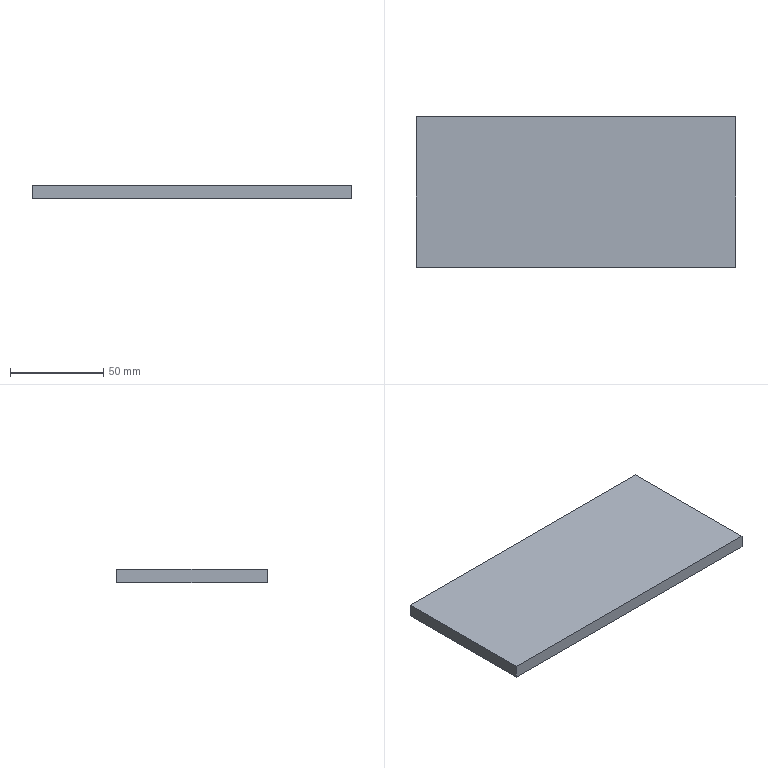Part | STEP file | 2026.6.15-Main Assembly图.sldasm-Part-108 | 1 solid | 6 faces | box 170.9 x 80.5 x 7 mm | volume 96302 mm3 | plane 6
STEP:
#1=CARTESIAN_POINT('',(-1674.674,519.051,4125.667));
#2=VERTEX_POINT('',#1);
#3=CARTESIAN_POINT('',(-1674.674,599.551,4125.667));
#4=VERTEX_POINT('',#3);
#5=CARTESIAN_POINT('',(-1674.674,519.051,4125.667));
#6=DIRECTION('',(0.,1.,0.));
#7=VECTOR('',#6,1000.);
#8=LINE('',#5,#7);
#9=EDGE_CURVE('',#2,#4,#8,.T.);
#10=ORIENTED_EDGE('',*,*,#9,.T.);
#11=CARTESIAN_POINT('',(-1674.674,599.551,4118.667));
#12=VERTEX_POINT('',#11);
#13=CARTESIAN_POINT('',(-1674.674,599.551,4118.667));
#14=DIRECTION('',(0.,0.,1.));
#15=VECTOR('',#14,1000.);
#16=LINE('',#13,#15);
#17=EDGE_CURVE('',#12,#4,#16,.T.);
#18=ORIENTED_EDGE('',*,*,#17,.F.);
#19=CARTESIAN_POINT('',(-1674.674,519.051,4118.667));
#20=VERTEX_POINT('',#19);
#21=CARTESIAN_POINT('',(-1674.674,519.051,4118.667));
#22=DIRECTION('',(0.,1.,0.));
#23=VECTOR('',#22,1000.);
#24=LINE('',#21,#23);
#25=EDGE_CURVE('',#20,#12,#24,.T.);
#26=ORIENTED_EDGE('',*,*,#25,.F.);
#27=CARTESIAN_POINT('',(-1674.674,519.051,4118.667));
#28=DIRECTION('',(0.,0.,1.));
#29=VECTOR('',#28,1000.);
#30=LINE('',#27,#29);
#31=EDGE_CURVE('',#20,#2,#30,.T.);
#32=ORIENTED_EDGE('',*,*,#31,.T.);
#33=EDGE_LOOP('',(#10,#18,#26,#32));
#34=FACE_OUTER_BOUND('',#33,.T.);
#35=CARTESIAN_POINT('',(-1674.674,519.051,4118.667));
#36=DIRECTION('',(1.,0.,0.));
#37=DIRECTION('',(0.,1.,0.));
#38=AXIS2_PLACEMENT_3D('',#35,#36,#37);
#39=PLANE('',#38);
#40=ADVANCED_FACE('',(#34),#39,.F.);
#41=CARTESIAN_POINT('',(-1503.774,599.551,4125.667));
#42=VERTEX_POINT('',#41);
#43=CARTESIAN_POINT('',(-1674.674,599.551,4125.667));
#44=DIRECTION('',(1.,0.,0.));
#45=VECTOR('',#44,1000.);
#46=LINE('',#43,#45);
#47=EDGE_CURVE('',#4,#42,#46,.T.);
#48=ORIENTED_EDGE('',*,*,#47,.T.);
#49=CARTESIAN_POINT('',(-1503.774,599.551,4118.667));
#50=VERTEX_POINT('',#49);
#51=CARTESIAN_POINT('',(-1503.774,599.551,4118.667));
#52=DIRECTION('',(0.,0.,1.));
#53=VECTOR('',#52,1000.);
#54=LINE('',#51,#53);
#55=EDGE_CURVE('',#50,#42,#54,.T.);
#56=ORIENTED_EDGE('',*,*,#55,.F.);
#57=CARTESIAN_POINT('',(-1674.674,599.551,4118.667));
#58=DIRECTION('',(1.,0.,0.));
#59=VECTOR('',#58,1000.);
#60=LINE('',#57,#59);
#61=EDGE_CURVE('',#12,#50,#60,.T.);
#62=ORIENTED_EDGE('',*,*,#61,.F.);
#63=ORIENTED_EDGE('',*,*,#17,.T.);
#64=EDGE_LOOP('',(#48,#56,#62,#63));
#65=FACE_OUTER_BOUND('',#64,.T.);
#66=CARTESIAN_POINT('',(-1674.674,599.551,4118.667));
#67=DIRECTION('',(0.,-1.,0.));
#68=DIRECTION('',(0.,0.,-1.));
#69=AXIS2_PLACEMENT_3D('',#66,#67,#68);
#70=PLANE('',#69);
#71=ADVANCED_FACE('',(#65),#70,.F.);
#72=CARTESIAN_POINT('',(-1503.774,519.051,4125.667));
#73=VERTEX_POINT('',#72);
#74=CARTESIAN_POINT('',(-1503.774,599.551,4125.667));
#75=DIRECTION('',(0.,-1.,0.));
#76=VECTOR('',#75,1000.);
#77=LINE('',#74,#76);
#78=EDGE_CURVE('',#42,#73,#77,.T.);
#79=ORIENTED_EDGE('',*,*,#78,.T.);
#80=CARTESIAN_POINT('',(-1503.774,519.051,4118.667));
#81=VERTEX_POINT('',#80);
#82=CARTESIAN_POINT('',(-1503.774,519.051,4118.667));
#83=DIRECTION('',(0.,0.,1.));
#84=VECTOR('',#83,1000.);
#85=LINE('',#82,#84);
#86=EDGE_CURVE('',#81,#73,#85,.T.);
#87=ORIENTED_EDGE('',*,*,#86,.F.);
#88=CARTESIAN_POINT('',(-1503.774,599.551,4118.667));
#89=DIRECTION('',(0.,-1.,0.));
#90=VECTOR('',#89,1000.);
#91=LINE('',#88,#90);
#92=EDGE_CURVE('',#50,#81,#91,.T.);
#93=ORIENTED_EDGE('',*,*,#92,.F.);
#94=ORIENTED_EDGE('',*,*,#55,.T.);
#95=EDGE_LOOP('',(#79,#87,#93,#94));
#96=FACE_OUTER_BOUND('',#95,.T.);
#97=CARTESIAN_POINT('',(-1503.774,599.551,4118.667));
#98=DIRECTION('',(-1.,0.,0.));
#99=DIRECTION('',(0.,-1.,0.));
#100=AXIS2_PLACEMENT_3D('',#97,#98,#99);
#101=PLANE('',#100);
#102=ADVANCED_FACE('',(#96),#101,.F.);
#103=CARTESIAN_POINT('',(-1503.774,519.051,4125.667));
#104=DIRECTION('',(-1.,0.,0.));
#105=VECTOR('',#104,1000.);
#106=LINE('',#103,#105);
#107=EDGE_CURVE('',#73,#2,#106,.T.);
#108=ORIENTED_EDGE('',*,*,#107,.T.);
#109=ORIENTED_EDGE('',*,*,#31,.F.);
#110=CARTESIAN_POINT('',(-1503.774,519.051,4118.667));
#111=DIRECTION('',(-1.,0.,0.));
#112=VECTOR('',#111,1000.);
#113=LINE('',#110,#112);
#114=EDGE_CURVE('',#81,#20,#113,.T.);
#115=ORIENTED_EDGE('',*,*,#114,.F.);
#116=ORIENTED_EDGE('',*,*,#86,.T.);
#117=EDGE_LOOP('',(#108,#109,#115,#116));
#118=FACE_OUTER_BOUND('',#117,.T.);
#119=CARTESIAN_POINT('',(-1503.774,519.051,4118.667));
#120=DIRECTION('',(0.,1.,0.));
#121=DIRECTION('',(0.,0.,1.));
#122=AXIS2_PLACEMENT_3D('',#119,#120,#121);
#123=PLANE('',#122);
#124=ADVANCED_FACE('',(#118),#123,.F.);
#125=ORIENTED_EDGE('',*,*,#25,.T.);
#126=ORIENTED_EDGE('',*,*,#61,.T.);
#127=ORIENTED_EDGE('',*,*,#92,.T.);
#128=ORIENTED_EDGE('',*,*,#114,.T.);
#129=EDGE_LOOP('',(#125,#126,#127,#128));
#130=FACE_OUTER_BOUND('',#129,.T.);
#131=CARTESIAN_POINT('',(-1612.964,406.261,4118.667));
#132=DIRECTION('',(0.,0.,-1.));
#133=DIRECTION('',(0.,1.,0.));
#134=AXIS2_PLACEMENT_3D('',#131,#132,#133);
#135=PLANE('',#134);
#136=ADVANCED_FACE('',(#130),#135,.T.);
#137=ORIENTED_EDGE('',*,*,#9,.F.);
#138=ORIENTED_EDGE('',*,*,#107,.F.);
#139=ORIENTED_EDGE('',*,*,#78,.F.);
#140=ORIENTED_EDGE('',*,*,#47,.F.);
#141=EDGE_LOOP('',(#137,#138,#139,#140));
#142=FACE_OUTER_BOUND('',#141,.T.);
#143=CARTESIAN_POINT('',(-1612.964,406.261,4125.667));
#144=DIRECTION('',(0.,0.,-1.));
#145=DIRECTION('',(0.,1.,0.));
#146=AXIS2_PLACEMENT_3D('',#143,#144,#145);
#147=PLANE('',#146);
#148=ADVANCED_FACE('',(#142),#147,.F.);
#149=CLOSED_SHELL('',(#40,#71,#102,#124,#136,#148));
#150=MANIFOLD_SOLID_BREP('',#149);
#151=CARTESIAN_POINT('',(0.,0.,0.));
#152=DIRECTION('',(0.,0.,1.));
#153=DIRECTION('',(1.,0.,0.));
#154=AXIS2_PLACEMENT_3D('',#151,#152,#153);
#155=(LENGTH_UNIT()NAMED_UNIT(*)SI_UNIT(.MILLI.,.METRE.));
#156=UNCERTAINTY_MEASURE_WITH_UNIT(LENGTH_MEASURE(0.00001),#155,'','');
#157=(NAMED_UNIT(*)PLANE_ANGLE_UNIT()SI_UNIT($,.RADIAN.));
#158=(NAMED_UNIT(*)SI_UNIT($,.STERADIAN.)SOLID_ANGLE_UNIT());
#159=(GEOMETRIC_REPRESENTATION_CONTEXT(3)GLOBAL_UNCERTAINTY_ASSIGNED_CONTEXT((#156))GLOBAL_UNIT_ASSIGNED_CONTEXT((#155,#157,#158))REPRESENTATION_CONTEXT('',''));
#160=ADVANCED_BREP_SHAPE_REPRESENTATION('',(#150,#154),#159);